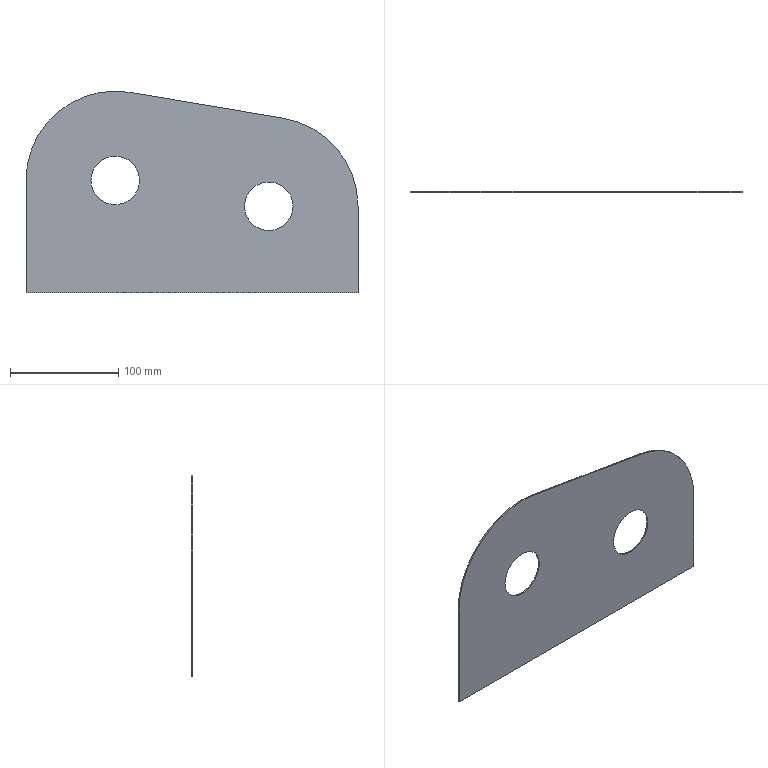Part | STEP file | 冲床-300配套压波_id410_x_t | 1 solid | 10 faces | box 307 x 1.2 x 186.5 mm | volume 57177 mm3 | plane 6 | cylinder 4 | commonest cylinder face diameters 45 x2 165 x2
STEP:
#1=CARTESIAN_POINT('',(1414.5,133.8,80.083));
#2=VERTEX_POINT('',#1);
#3=CARTESIAN_POINT('',(1392.,133.8,80.083));
#4=DIRECTION('',(0.,1.,0.));
#5=DIRECTION('',(1.,0.,0.));
#6=AXIS2_PLACEMENT_3D('',#3,#4,#5);
#7=CIRCLE('',#6,22.5);
#8=EDGE_CURVE('',#2,#2,#7,.T.);
#9=ORIENTED_EDGE('',*,*,#8,.F.);
#10=EDGE_LOOP('',(#9));
#11=FACE_BOUND('',#10,.T.);
#12=CARTESIAN_POINT('',(1369.5,135.,80.083));
#13=VERTEX_POINT('',#12);
#14=CARTESIAN_POINT('',(1392.,135.,80.083));
#15=DIRECTION('',(0.,1.,0.));
#16=DIRECTION('',(-1.,0.,0.));
#17=AXIS2_PLACEMENT_3D('',#14,#15,#16);
#18=CIRCLE('',#17,22.5);
#19=EDGE_CURVE('',#13,#13,#18,.T.);
#20=ORIENTED_EDGE('',*,*,#19,.T.);
#21=EDGE_LOOP('',(#20));
#22=FACE_BOUND('',#21,.T.);
#23=CARTESIAN_POINT('',(1392.,49.5,80.083));
#24=DIRECTION('',(0.,1.,0.));
#25=DIRECTION('',(0.,0.,1.));
#26=AXIS2_PLACEMENT_3D('',#23,#24,#25);
#27=CYLINDRICAL_SURFACE('',#26,22.5);
#28=ADVANCED_FACE('',(#11,#22),#27,.F.);
#29=CARTESIAN_POINT('',(1227.5,135.,104.));
#30=VERTEX_POINT('',#29);
#31=CARTESIAN_POINT('',(1250.,135.,104.));
#32=DIRECTION('',(0.,-1.,0.));
#33=DIRECTION('',(-1.,0.,0.));
#34=AXIS2_PLACEMENT_3D('',#31,#32,#33);
#35=CIRCLE('',#34,22.5);
#36=EDGE_CURVE('',#30,#30,#35,.T.);
#37=ORIENTED_EDGE('',*,*,#36,.F.);
#38=EDGE_LOOP('',(#37));
#39=FACE_BOUND('',#38,.T.);
#40=CARTESIAN_POINT('',(1272.5,133.8,104.));
#41=VERTEX_POINT('',#40);
#42=CARTESIAN_POINT('',(1250.,133.8,104.));
#43=DIRECTION('',(0.,1.,0.));
#44=DIRECTION('',(1.,0.,0.));
#45=AXIS2_PLACEMENT_3D('',#42,#43,#44);
#46=CIRCLE('',#45,22.5);
#47=EDGE_CURVE('',#41,#41,#46,.T.);
#48=ORIENTED_EDGE('',*,*,#47,.F.);
#49=EDGE_LOOP('',(#48));
#50=FACE_BOUND('',#49,.T.);
#51=CARTESIAN_POINT('',(1250.,140.,104.));
#52=DIRECTION('',(0.,-1.,0.));
#53=DIRECTION('',(-1.,0.,0.));
#54=AXIS2_PLACEMENT_3D('',#51,#52,#53);
#55=CYLINDRICAL_SURFACE('',#54,22.5);
#56=ADVANCED_FACE('',(#39,#50),#55,.F.);
#57=CARTESIAN_POINT('',(1474.5,135.,0.));
#58=VERTEX_POINT('',#57);
#59=CARTESIAN_POINT('',(1474.5,133.8,0.));
#60=VERTEX_POINT('',#59);
#61=CARTESIAN_POINT('',(1474.5,71.5,0.));
#62=DIRECTION('',(0.,-1.,0.));
#63=VECTOR('',#62,1.);
#64=LINE('',#61,#63);
#65=EDGE_CURVE('',#58,#60,#64,.T.);
#66=ORIENTED_EDGE('',*,*,#65,.T.);
#67=CARTESIAN_POINT('',(1167.5,133.8,0.));
#68=VERTEX_POINT('',#67);
#69=CARTESIAN_POINT('',(1507.,133.8,0.));
#70=DIRECTION('',(1.,0.,0.));
#71=VECTOR('',#70,1.);
#72=LINE('',#69,#71);
#73=EDGE_CURVE('',#68,#60,#72,.T.);
#74=ORIENTED_EDGE('',*,*,#73,.F.);
#75=CARTESIAN_POINT('',(1167.5,135.,0.));
#76=VERTEX_POINT('',#75);
#77=CARTESIAN_POINT('',(1167.5,71.5,0.));
#78=DIRECTION('',(0.,1.,0.));
#79=VECTOR('',#78,1.);
#80=LINE('',#77,#79);
#81=EDGE_CURVE('',#68,#76,#80,.T.);
#82=ORIENTED_EDGE('',*,*,#81,.T.);
#83=CARTESIAN_POINT('',(1507.,135.,0.));
#84=DIRECTION('',(1.,0.,0.));
#85=VECTOR('',#84,1.);
#86=LINE('',#83,#85);
#87=EDGE_CURVE('',#76,#58,#86,.T.);
#88=ORIENTED_EDGE('',*,*,#87,.T.);
#89=EDGE_LOOP('',(#66,#74,#82,#88));
#90=FACE_OUTER_BOUND('',#89,.T.);
#91=CARTESIAN_POINT('',(1507.,71.5,0.));
#92=DIRECTION('',(0.,0.,1.));
#93=DIRECTION('',(1.,0.,0.));
#94=AXIS2_PLACEMENT_3D('',#91,#92,#93);
#95=PLANE('',#94);
#96=ADVANCED_FACE('',(#90),#95,.F.);
#97=ORIENTED_EDGE('',*,*,#8,.T.);
#98=EDGE_LOOP('',(#97));
#99=FACE_BOUND('',#98,.T.);
#100=ORIENTED_EDGE('',*,*,#47,.T.);
#101=EDGE_LOOP('',(#100));
#102=FACE_BOUND('',#101,.T.);
#103=ORIENTED_EDGE('',*,*,#73,.T.);
#104=CARTESIAN_POINT('',(1474.5,133.8,80.083));
#105=VERTEX_POINT('',#104);
#106=CARTESIAN_POINT('',(1474.5,133.8,0.));
#107=DIRECTION('',(0.,0.,-1.));
#108=VECTOR('',#107,1.);
#109=LINE('',#106,#108);
#110=EDGE_CURVE('',#105,#60,#109,.T.);
#111=ORIENTED_EDGE('',*,*,#110,.F.);
#112=CARTESIAN_POINT('',(1405.702,133.8,161.438));
#113=VERTEX_POINT('',#112);
#114=CARTESIAN_POINT('',(1392.,133.8,80.083));
#115=DIRECTION('',(0.,1.,0.));
#116=DIRECTION('',(1.,0.,0.));
#117=AXIS2_PLACEMENT_3D('',#114,#115,#116);
#118=CIRCLE('',#117,82.5);
#119=EDGE_CURVE('',#113,#105,#118,.T.);
#120=ORIENTED_EDGE('',*,*,#119,.F.);
#121=CARTESIAN_POINT('',(1263.702,133.8,185.354));
#122=VERTEX_POINT('',#121);
#123=CARTESIAN_POINT('',(1263.702,133.8,185.354));
#124=DIRECTION('',(-0.9861,0.,0.1661));
#125=VECTOR('',#124,1.);
#126=LINE('',#123,#125);
#127=EDGE_CURVE('',#113,#122,#126,.T.);
#128=ORIENTED_EDGE('',*,*,#127,.T.);
#129=CARTESIAN_POINT('',(1167.5,133.8,104.));
#130=VERTEX_POINT('',#129);
#131=CARTESIAN_POINT('',(1250.,133.8,104.));
#132=DIRECTION('',(0.,-1.,0.));
#133=DIRECTION('',(1.,0.,0.));
#134=AXIS2_PLACEMENT_3D('',#131,#132,#133);
#135=CIRCLE('',#134,82.5);
#136=EDGE_CURVE('',#122,#130,#135,.T.);
#137=ORIENTED_EDGE('',*,*,#136,.T.);
#138=CARTESIAN_POINT('',(1167.5,133.8,360.));
#139=DIRECTION('',(0.,0.,-1.));
#140=VECTOR('',#139,1.);
#141=LINE('',#138,#140);
#142=EDGE_CURVE('',#130,#68,#141,.T.);
#143=ORIENTED_EDGE('',*,*,#142,.T.);
#144=EDGE_LOOP('',(#103,#111,#120,#128,#137,#143));
#145=FACE_BOUND('',#144,.T.);
#146=CARTESIAN_POINT('',(1165.,133.8,360.));
#147=DIRECTION('',(0.,-1.,0.));
#148=DIRECTION('',(0.,0.,1.));
#149=AXIS2_PLACEMENT_3D('',#146,#147,#148);
#150=PLANE('',#149);
#151=ADVANCED_FACE('',(#99,#102,#145),#150,.T.);
#152=CARTESIAN_POINT('',(1167.5,135.,104.));
#153=VERTEX_POINT('',#152);
#154=CARTESIAN_POINT('',(1167.5,135.,104.));
#155=DIRECTION('',(0.,0.,1.));
#156=VECTOR('',#155,1.);
#157=LINE('',#154,#156);
#158=EDGE_CURVE('',#76,#153,#157,.T.);
#159=ORIENTED_EDGE('',*,*,#158,.T.);
#160=CARTESIAN_POINT('',(1263.702,135.,185.354));
#161=VERTEX_POINT('',#160);
#162=CARTESIAN_POINT('',(1250.,135.,104.));
#163=DIRECTION('',(0.,-1.,0.));
#164=DIRECTION('',(-1.,0.,0.));
#165=AXIS2_PLACEMENT_3D('',#162,#163,#164);
#166=CIRCLE('',#165,82.5);
#167=EDGE_CURVE('',#161,#153,#166,.T.);
#168=ORIENTED_EDGE('',*,*,#167,.F.);
#169=CARTESIAN_POINT('',(1405.702,135.,161.438));
#170=VERTEX_POINT('',#169);
#171=CARTESIAN_POINT('',(1263.702,135.,185.354));
#172=DIRECTION('',(-0.9861,0.,0.1661));
#173=VECTOR('',#172,1.);
#174=LINE('',#171,#173);
#175=EDGE_CURVE('',#170,#161,#174,.T.);
#176=ORIENTED_EDGE('',*,*,#175,.F.);
#177=CARTESIAN_POINT('',(1474.5,135.,80.083));
#178=VERTEX_POINT('',#177);
#179=CARTESIAN_POINT('',(1392.,135.,80.083));
#180=DIRECTION('',(0.,-1.,0.));
#181=DIRECTION('',(-1.,0.,0.));
#182=AXIS2_PLACEMENT_3D('',#179,#180,#181);
#183=CIRCLE('',#182,82.5);
#184=EDGE_CURVE('',#178,#170,#183,.T.);
#185=ORIENTED_EDGE('',*,*,#184,.F.);
#186=CARTESIAN_POINT('',(1474.5,135.,104.));
#187=DIRECTION('',(0.,0.,-1.));
#188=VECTOR('',#187,1.);
#189=LINE('',#186,#188);
#190=EDGE_CURVE('',#178,#58,#189,.T.);
#191=ORIENTED_EDGE('',*,*,#190,.T.);
#192=ORIENTED_EDGE('',*,*,#87,.F.);
#193=EDGE_LOOP('',(#159,#168,#176,#185,#191,#192));
#194=FACE_BOUND('',#193,.T.);
#195=ORIENTED_EDGE('',*,*,#36,.T.);
#196=EDGE_LOOP('',(#195));
#197=FACE_BOUND('',#196,.T.);
#198=ORIENTED_EDGE('',*,*,#19,.F.);
#199=EDGE_LOOP('',(#198));
#200=FACE_BOUND('',#199,.T.);
#201=CARTESIAN_POINT('',(1250.,135.,104.));
#202=DIRECTION('',(0.,1.,0.));
#203=DIRECTION('',(0.9861,0.,-0.1661));
#204=AXIS2_PLACEMENT_3D('',#201,#202,#203);
#205=PLANE('',#204);
#206=ADVANCED_FACE('',(#194,#197,#200),#205,.T.);
#207=ORIENTED_EDGE('',*,*,#158,.F.);
#208=ORIENTED_EDGE('',*,*,#81,.F.);
#209=ORIENTED_EDGE('',*,*,#142,.F.);
#210=CARTESIAN_POINT('',(1167.5,400.5,104.));
#211=DIRECTION('',(0.,-1.,0.));
#212=VECTOR('',#211,1.);
#213=LINE('',#210,#212);
#214=EDGE_CURVE('',#153,#130,#213,.T.);
#215=ORIENTED_EDGE('',*,*,#214,.F.);
#216=EDGE_LOOP('',(#207,#208,#209,#215));
#217=FACE_OUTER_BOUND('',#216,.T.);
#218=CARTESIAN_POINT('',(1167.5,-133.,104.));
#219=DIRECTION('',(-1.,0.,0.));
#220=DIRECTION('',(0.,0.,1.));
#221=AXIS2_PLACEMENT_3D('',#218,#219,#220);
#222=PLANE('',#221);
#223=ADVANCED_FACE('',(#217),#222,.T.);
#224=ORIENTED_EDGE('',*,*,#110,.T.);
#225=ORIENTED_EDGE('',*,*,#65,.F.);
#226=ORIENTED_EDGE('',*,*,#190,.F.);
#227=CARTESIAN_POINT('',(1474.5,400.5,80.083));
#228=DIRECTION('',(0.,-1.,0.));
#229=VECTOR('',#228,1.);
#230=LINE('',#227,#229);
#231=EDGE_CURVE('',#178,#105,#230,.T.);
#232=ORIENTED_EDGE('',*,*,#231,.T.);
#233=EDGE_LOOP('',(#224,#225,#226,#232));
#234=FACE_OUTER_BOUND('',#233,.T.);
#235=CARTESIAN_POINT('',(1474.5,-133.,0.));
#236=DIRECTION('',(1.,0.,0.));
#237=DIRECTION('',(0.,0.,-1.));
#238=AXIS2_PLACEMENT_3D('',#235,#236,#237);
#239=PLANE('',#238);
#240=ADVANCED_FACE('',(#234),#239,.T.);
#241=CARTESIAN_POINT('',(1405.702,400.5,161.438));
#242=DIRECTION('',(0.,1.,0.));
#243=VECTOR('',#242,1.);
#244=LINE('',#241,#243);
#245=EDGE_CURVE('',#113,#170,#244,.T.);
#246=ORIENTED_EDGE('',*,*,#245,.T.);
#247=ORIENTED_EDGE('',*,*,#175,.T.);
#248=CARTESIAN_POINT('',(1263.702,400.5,185.354));
#249=DIRECTION('',(0.,1.,0.));
#250=VECTOR('',#249,1.);
#251=LINE('',#248,#250);
#252=EDGE_CURVE('',#122,#161,#251,.T.);
#253=ORIENTED_EDGE('',*,*,#252,.F.);
#254=ORIENTED_EDGE('',*,*,#127,.F.);
#255=EDGE_LOOP('',(#246,#247,#253,#254));
#256=FACE_OUTER_BOUND('',#255,.T.);
#257=CARTESIAN_POINT('',(1263.702,400.5,185.354));
#258=DIRECTION('',(-0.1661,0.,-0.9861));
#259=DIRECTION('',(-0.9861,0.,0.1661));
#260=AXIS2_PLACEMENT_3D('',#257,#258,#259);
#261=PLANE('',#260);
#262=ADVANCED_FACE('',(#256),#261,.F.);
#263=ORIENTED_EDGE('',*,*,#252,.T.);
#264=ORIENTED_EDGE('',*,*,#167,.T.);
#265=ORIENTED_EDGE('',*,*,#214,.T.);
#266=ORIENTED_EDGE('',*,*,#136,.F.);
#267=EDGE_LOOP('',(#263,#264,#265,#266));
#268=FACE_OUTER_BOUND('',#267,.T.);
#269=CARTESIAN_POINT('',(1250.,400.5,104.));
#270=DIRECTION('',(0.,-1.,0.));
#271=DIRECTION('',(1.,0.,0.));
#272=AXIS2_PLACEMENT_3D('',#269,#270,#271);
#273=CYLINDRICAL_SURFACE('',#272,82.5);
#274=ADVANCED_FACE('',(#268),#273,.T.);
#275=ORIENTED_EDGE('',*,*,#119,.T.);
#276=ORIENTED_EDGE('',*,*,#231,.F.);
#277=ORIENTED_EDGE('',*,*,#184,.T.);
#278=ORIENTED_EDGE('',*,*,#245,.F.);
#279=EDGE_LOOP('',(#275,#276,#277,#278));
#280=FACE_OUTER_BOUND('',#279,.T.);
#281=CARTESIAN_POINT('',(1392.,400.5,80.083));
#282=DIRECTION('',(0.,-1.,0.));
#283=DIRECTION('',(1.,0.,0.));
#284=AXIS2_PLACEMENT_3D('',#281,#282,#283);
#285=CYLINDRICAL_SURFACE('',#284,82.5);
#286=ADVANCED_FACE('',(#280),#285,.T.);
#287=CLOSED_SHELL('',(#28,#56,#96,#151,#206,#223,#240,#262,#274,#286));
#288=MANIFOLD_SOLID_BREP('',#287);
#289=(LENGTH_UNIT()NAMED_UNIT(*)SI_UNIT(.MILLI.,.METRE.));
#290=UNCERTAINTY_MEASURE_WITH_UNIT(LENGTH_MEASURE(0.00002),#289,'','');
#291=(NAMED_UNIT(*)PLANE_ANGLE_UNIT()SI_UNIT($,.RADIAN.));
#292=PLANE_ANGLE_MEASURE_WITH_UNIT(PLANE_ANGLE_MEASURE(0.01745),#291);
#293=DIMENSIONAL_EXPONENTS(0.,0.,0.,0.,0.,0.,0.);
#294=(CONVERSION_BASED_UNIT('DEGREE',#292)NAMED_UNIT(#293)PLANE_ANGLE_UNIT());
#295=(NAMED_UNIT(*)SI_UNIT($,.STERADIAN.)SOLID_ANGLE_UNIT());
#296=(GEOMETRIC_REPRESENTATION_CONTEXT(3)GLOBAL_UNCERTAINTY_ASSIGNED_CONTEXT((#290))GLOBAL_UNIT_ASSIGNED_CONTEXT((#289,#294,#295))REPRESENTATION_CONTEXT('',''));
#297=ADVANCED_BREP_SHAPE_REPRESENTATION('',(#288),#296);